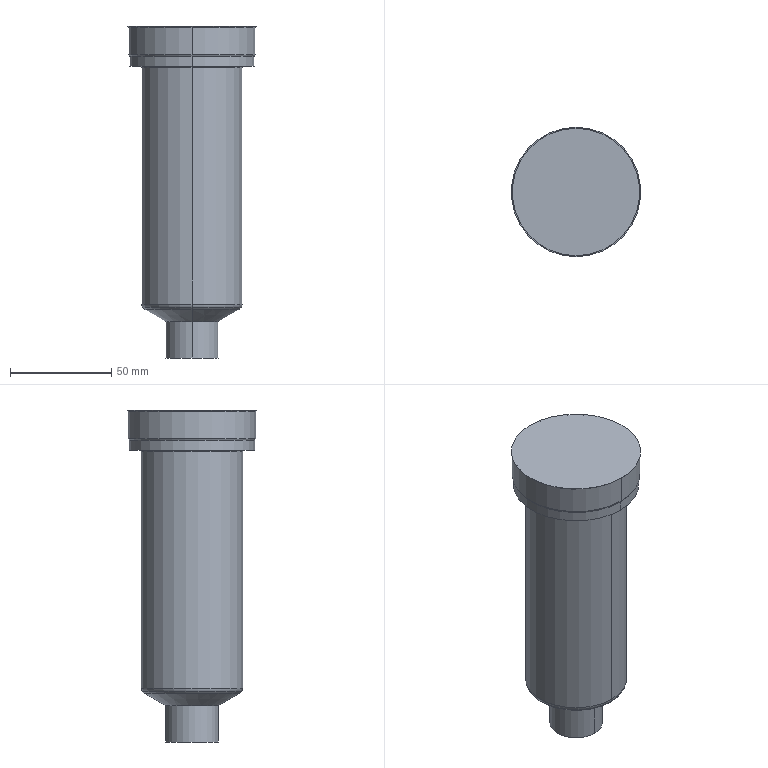Part | Creo | 1 solid | 23 faces | box 64 x 64 x 164.09 mm | volume 313430 mm3 | cylinder 8 | cone 8 | torus 4 | plane 3 | commonest cylinder face diameters 26 x2 50 x2 62 x2 63 x2
STEP:
#1=CARTESIAN_POINT('',(0.,48.,36.41));
#2=VERTEX_POINT('',#1);
#3=CARTESIAN_POINT('',(0.,22.,36.41));
#4=VERTEX_POINT('',#3);
#5=CARTESIAN_POINT('',(0.,35.,36.41));
#6=DIRECTION('',(0.,0.,-1.));
#7=DIRECTION('',(0.,1.,0.));
#8=AXIS2_PLACEMENT_3D('',#5,#6,#7);
#9=CIRCLE('',#8,13.);
#10=EDGE_CURVE('',#2,#4,#9,.T.);
#11=ORIENTED_EDGE('',*,*,#10,.F.);
#12=CARTESIAN_POINT('',(0.,35.,36.41));
#13=DIRECTION('',(0.,0.,-1.));
#14=DIRECTION('',(0.,-1.,0.));
#15=AXIS2_PLACEMENT_3D('',#12,#13,#14);
#16=CIRCLE('',#15,13.);
#17=EDGE_CURVE('',#4,#2,#16,.T.);
#18=ORIENTED_EDGE('',*,*,#17,.F.);
#19=EDGE_LOOP('',(#11,#18));
#20=FACE_OUTER_BOUND('',#19,.F.);
#21=CARTESIAN_POINT('',(1.,35.,36.41));
#22=DIRECTION('',(0.,0.,-1.));
#23=DIRECTION('',(0.,1.,0.));
#24=AXIS2_PLACEMENT_3D('',#21,#22,#23);
#25=PLANE('',#24);
#26=ADVANCED_FACE('',(#20),#25,.T.);
#27=CARTESIAN_POINT('',(0.,22.,54.41));
#28=VERTEX_POINT('',#27);
#29=CARTESIAN_POINT('',(0.,48.,54.41));
#30=VERTEX_POINT('',#29);
#31=CARTESIAN_POINT('',(0.,35.,54.41));
#32=DIRECTION('',(0.,0.,1.));
#33=DIRECTION('',(0.,-1.,0.));
#34=AXIS2_PLACEMENT_3D('',#31,#32,#33);
#35=CIRCLE('',#34,13.);
#36=EDGE_CURVE('',#28,#30,#35,.T.);
#37=ORIENTED_EDGE('',*,*,#36,.T.);
#38=CARTESIAN_POINT('',(0.,48.,54.41));
#39=DIRECTION('',(0.,0.,-1.));
#40=VECTOR('',#39,18.);
#41=LINE('',#38,#40);
#42=EDGE_CURVE('',#30,#2,#41,.T.);
#43=ORIENTED_EDGE('',*,*,#42,.T.);
#44=ORIENTED_EDGE('',*,*,#10,.T.);
#45=CARTESIAN_POINT('',(0.,22.,54.41));
#46=DIRECTION('',(0.,0.,-1.));
#47=VECTOR('',#46,18.);
#48=LINE('',#45,#47);
#49=EDGE_CURVE('',#28,#4,#48,.T.);
#50=ORIENTED_EDGE('',*,*,#49,.F.);
#51=EDGE_LOOP('',(#37,#43,#44,#50));
#52=FACE_OUTER_BOUND('',#51,.F.);
#53=CARTESIAN_POINT('',(0.,35.,36.41));
#54=DIRECTION('',(0.,0.,-1.));
#55=DIRECTION('',(0.,1.,0.));
#56=AXIS2_PLACEMENT_3D('',#53,#54,#55);
#57=CYLINDRICAL_SURFACE('',#56,13.);
#58=ADVANCED_FACE('',(#52),#57,.T.);
#59=CARTESIAN_POINT('',(0.,11.5,60.472));
#60=VERTEX_POINT('',#59);
#61=CARTESIAN_POINT('',(0.,58.5,60.472));
#62=VERTEX_POINT('',#61);
#63=CARTESIAN_POINT('',(0.,35.,60.472));
#64=DIRECTION('',(0.,0.,1.));
#65=DIRECTION('',(0.,-1.,0.));
#66=AXIS2_PLACEMENT_3D('',#63,#64,#65);
#67=CIRCLE('',#66,23.5);
#68=EDGE_CURVE('',#60,#62,#67,.T.);
#69=ORIENTED_EDGE('',*,*,#68,.T.);
#70=CARTESIAN_POINT('',(0.,48.,54.41));
#71=DIRECTION('',(0.,0.866,0.5));
#72=VECTOR('',#71,12.124);
#73=LINE('',#70,#72);
#74=EDGE_CURVE('',#30,#62,#73,.T.);
#75=ORIENTED_EDGE('',*,*,#74,.F.);
#76=ORIENTED_EDGE('',*,*,#36,.F.);
#77=CARTESIAN_POINT('',(0.,22.,54.41));
#78=DIRECTION('',(0.,-0.866,0.5));
#79=VECTOR('',#78,12.124);
#80=LINE('',#77,#79);
#81=EDGE_CURVE('',#28,#60,#80,.T.);
#82=ORIENTED_EDGE('',*,*,#81,.T.);
#83=EDGE_LOOP('',(#69,#75,#76,#82));
#84=FACE_OUTER_BOUND('',#83,.F.);
#85=CARTESIAN_POINT('',(0.,35.,57.441));
#86=DIRECTION('',(0.,0.,1.));
#87=DIRECTION('',(0.,-1.,0.));
#88=AXIS2_PLACEMENT_3D('',#85,#86,#87);
#89=CONICAL_SURFACE('',#88,18.25,60.);
#90=ADVANCED_FACE('',(#84),#89,.T.);
#91=ORIENTED_EDGE('',*,*,#68,.F.);
#92=CARTESIAN_POINT('',(0.,10.402,61.57));
#93=VERTEX_POINT('',#92);
#94=CARTESIAN_POINT('',(0.,13.,63.07));
#95=DIRECTION('',(1.,0.,0.));
#96=DIRECTION('',(0.,-0.866,-0.5));
#97=AXIS2_PLACEMENT_3D('',#94,#95,#96);
#98=CIRCLE('',#97,3.);
#99=EDGE_CURVE('',#93,#60,#98,.T.);
#100=ORIENTED_EDGE('',*,*,#99,.F.);
#101=CARTESIAN_POINT('',(0.,59.598,61.57));
#102=VERTEX_POINT('',#101);
#103=CARTESIAN_POINT('',(0.,35.,61.57));
#104=DIRECTION('',(0.,0.,-1.));
#105=DIRECTION('',(0.,1.,0.));
#106=AXIS2_PLACEMENT_3D('',#103,#104,#105);
#107=CIRCLE('',#106,24.598);
#108=EDGE_CURVE('',#102,#93,#107,.T.);
#109=ORIENTED_EDGE('',*,*,#108,.F.);
#110=CARTESIAN_POINT('',(0.,57.,63.07));
#111=DIRECTION('',(-1.,0.,0.));
#112=DIRECTION('',(0.,0.866,-0.5));
#113=AXIS2_PLACEMENT_3D('',#110,#111,#112);
#114=CIRCLE('',#113,3.);
#115=EDGE_CURVE('',#102,#62,#114,.T.);
#116=ORIENTED_EDGE('',*,*,#115,.T.);
#117=EDGE_LOOP('',(#91,#100,#109,#116));
#118=FACE_OUTER_BOUND('',#117,.F.);
#119=CARTESIAN_POINT('',(0.,35.,63.07));
#120=DIRECTION('',(0.,0.,-1.));
#121=DIRECTION('',(0.,1.,0.));
#122=AXIS2_PLACEMENT_3D('',#119,#120,#121);
#123=TOROIDAL_SURFACE('',#122,22.,3.);
#124=ADVANCED_FACE('',(#118),#123,.T.);
#125=CARTESIAN_POINT('',(0.,35.,60.472));
#126=DIRECTION('',(0.,0.,1.));
#127=DIRECTION('',(0.,1.,0.));
#128=AXIS2_PLACEMENT_3D('',#125,#126,#127);
#129=CIRCLE('',#128,23.5);
#130=EDGE_CURVE('',#62,#60,#129,.T.);
#131=ORIENTED_EDGE('',*,*,#130,.F.);
#132=ORIENTED_EDGE('',*,*,#115,.F.);
#133=CARTESIAN_POINT('',(0.,35.,61.57));
#134=DIRECTION('',(0.,0.,-1.));
#135=DIRECTION('',(0.,-1.,0.));
#136=AXIS2_PLACEMENT_3D('',#133,#134,#135);
#137=CIRCLE('',#136,24.598);
#138=EDGE_CURVE('',#93,#102,#137,.T.);
#139=ORIENTED_EDGE('',*,*,#138,.F.);
#140=ORIENTED_EDGE('',*,*,#99,.T.);
#141=EDGE_LOOP('',(#131,#132,#139,#140));
#142=FACE_OUTER_BOUND('',#141,.F.);
#143=CARTESIAN_POINT('',(0.,35.,63.07));
#144=DIRECTION('',(0.,0.,-1.));
#145=DIRECTION('',(0.,1.,0.));
#146=AXIS2_PLACEMENT_3D('',#143,#144,#145);
#147=TOROIDAL_SURFACE('',#146,22.,3.);
#148=ADVANCED_FACE('',(#142),#147,.T.);
#149=ORIENTED_EDGE('',*,*,#130,.T.);
#150=ORIENTED_EDGE('',*,*,#81,.F.);
#151=CARTESIAN_POINT('',(0.,35.,54.41));
#152=DIRECTION('',(0.,0.,1.));
#153=DIRECTION('',(0.,1.,0.));
#154=AXIS2_PLACEMENT_3D('',#151,#152,#153);
#155=CIRCLE('',#154,13.);
#156=EDGE_CURVE('',#30,#28,#155,.T.);
#157=ORIENTED_EDGE('',*,*,#156,.F.);
#158=ORIENTED_EDGE('',*,*,#74,.T.);
#159=EDGE_LOOP('',(#149,#150,#157,#158));
#160=FACE_OUTER_BOUND('',#159,.F.);
#161=CARTESIAN_POINT('',(0.,35.,57.441));
#162=DIRECTION('',(0.,0.,1.));
#163=DIRECTION('',(0.,-1.,0.));
#164=AXIS2_PLACEMENT_3D('',#161,#162,#163);
#165=CONICAL_SURFACE('',#164,18.25,60.);
#166=ADVANCED_FACE('',(#160),#165,.T.);
#167=ORIENTED_EDGE('',*,*,#156,.T.);
#168=ORIENTED_EDGE('',*,*,#49,.T.);
#169=ORIENTED_EDGE('',*,*,#17,.T.);
#170=ORIENTED_EDGE('',*,*,#42,.F.);
#171=EDGE_LOOP('',(#167,#168,#169,#170));
#172=FACE_OUTER_BOUND('',#171,.F.);
#173=CARTESIAN_POINT('',(0.,35.,36.41));
#174=DIRECTION('',(0.,0.,-1.));
#175=DIRECTION('',(0.,1.,0.));
#176=AXIS2_PLACEMENT_3D('',#173,#174,#175);
#177=CYLINDRICAL_SURFACE('',#176,13.);
#178=ADVANCED_FACE('',(#172),#177,.T.);
#179=CARTESIAN_POINT('',(0.,10.,63.07));
#180=VERTEX_POINT('',#179);
#181=CARTESIAN_POINT('',(0.,60.,63.07));
#182=VERTEX_POINT('',#181);
#183=CARTESIAN_POINT('',(0.,35.,63.07));
#184=DIRECTION('',(0.,0.,-1.));
#185=DIRECTION('',(0.,-1.,0.));
#186=AXIS2_PLACEMENT_3D('',#183,#184,#185);
#187=CIRCLE('',#186,25.);
#188=EDGE_CURVE('',#180,#182,#187,.T.);
#189=ORIENTED_EDGE('',*,*,#188,.F.);
#190=CARTESIAN_POINT('',(0.,13.,63.07));
#191=DIRECTION('',(1.,0.,0.));
#192=DIRECTION('',(0.,-1.,0.));
#193=AXIS2_PLACEMENT_3D('',#190,#191,#192);
#194=CIRCLE('',#193,3.);
#195=EDGE_CURVE('',#180,#93,#194,.T.);
#196=ORIENTED_EDGE('',*,*,#195,.T.);
#197=ORIENTED_EDGE('',*,*,#138,.T.);
#198=CARTESIAN_POINT('',(0.,57.,63.07));
#199=DIRECTION('',(-1.,0.,0.));
#200=DIRECTION('',(0.,1.,0.));
#201=AXIS2_PLACEMENT_3D('',#198,#199,#200);
#202=CIRCLE('',#201,3.);
#203=EDGE_CURVE('',#182,#102,#202,.T.);
#204=ORIENTED_EDGE('',*,*,#203,.F.);
#205=EDGE_LOOP('',(#189,#196,#197,#204));
#206=FACE_OUTER_BOUND('',#205,.F.);
#207=CARTESIAN_POINT('',(0.,35.,63.07));
#208=DIRECTION('',(0.,0.,-1.));
#209=DIRECTION('',(0.,1.,0.));
#210=AXIS2_PLACEMENT_3D('',#207,#208,#209);
#211=TOROIDAL_SURFACE('',#210,22.,3.);
#212=ADVANCED_FACE('',(#206),#211,.T.);
#213=CARTESIAN_POINT('',(0.,60.,180.));
#214=VERTEX_POINT('',#213);
#215=CARTESIAN_POINT('',(0.,10.,180.));
#216=VERTEX_POINT('',#215);
#217=CARTESIAN_POINT('',(0.,35.,180.));
#218=DIRECTION('',(0.,0.,1.));
#219=DIRECTION('',(0.,1.,0.));
#220=AXIS2_PLACEMENT_3D('',#217,#218,#219);
#221=CIRCLE('',#220,25.);
#222=EDGE_CURVE('',#214,#216,#221,.T.);
#223=ORIENTED_EDGE('',*,*,#222,.T.);
#224=CARTESIAN_POINT('',(0.,10.,180.));
#225=DIRECTION('',(0.,0.,-1.));
#226=VECTOR('',#225,116.93);
#227=LINE('',#224,#226);
#228=EDGE_CURVE('',#216,#180,#227,.T.);
#229=ORIENTED_EDGE('',*,*,#228,.T.);
#230=ORIENTED_EDGE('',*,*,#188,.T.);
#231=CARTESIAN_POINT('',(0.,60.,180.));
#232=DIRECTION('',(0.,0.,-1.));
#233=VECTOR('',#232,116.93);
#234=LINE('',#231,#233);
#235=EDGE_CURVE('',#214,#182,#234,.T.);
#236=ORIENTED_EDGE('',*,*,#235,.F.);
#237=EDGE_LOOP('',(#223,#229,#230,#236));
#238=FACE_OUTER_BOUND('',#237,.F.);
#239=CARTESIAN_POINT('',(0.,35.,36.41));
#240=DIRECTION('',(0.,0.,-1.));
#241=DIRECTION('',(0.,1.,0.));
#242=AXIS2_PLACEMENT_3D('',#239,#240,#241);
#243=CYLINDRICAL_SURFACE('',#242,25.);
#244=ADVANCED_FACE('',(#238),#243,.T.);
#245=CARTESIAN_POINT('',(0.,60.5,180.5));
#246=VERTEX_POINT('',#245);
#247=CARTESIAN_POINT('',(0.,9.5,180.5));
#248=VERTEX_POINT('',#247);
#249=CARTESIAN_POINT('',(0.,35.,180.5));
#250=DIRECTION('',(0.,0.,1.));
#251=DIRECTION('',(0.,1.,0.));
#252=AXIS2_PLACEMENT_3D('',#249,#250,#251);
#253=CIRCLE('',#252,25.5);
#254=EDGE_CURVE('',#246,#248,#253,.T.);
#255=ORIENTED_EDGE('',*,*,#254,.T.);
#256=CARTESIAN_POINT('',(0.,10.,180.));
#257=DIRECTION('',(0.,-0.7071,0.7071));
#258=VECTOR('',#257,0.7071);
#259=LINE('',#256,#258);
#260=EDGE_CURVE('',#216,#248,#259,.T.);
#261=ORIENTED_EDGE('',*,*,#260,.F.);
#262=ORIENTED_EDGE('',*,*,#222,.F.);
#263=CARTESIAN_POINT('',(0.,60.,180.));
#264=DIRECTION('',(0.,0.7071,0.7071));
#265=VECTOR('',#264,0.7071);
#266=LINE('',#263,#265);
#267=EDGE_CURVE('',#214,#246,#266,.T.);
#268=ORIENTED_EDGE('',*,*,#267,.T.);
#269=EDGE_LOOP('',(#255,#261,#262,#268));
#270=FACE_OUTER_BOUND('',#269,.F.);
#271=CARTESIAN_POINT('',(0.,35.,180.25));
#272=DIRECTION('',(0.,0.,1.));
#273=DIRECTION('',(0.,-1.,0.));
#274=AXIS2_PLACEMENT_3D('',#271,#272,#273);
#275=CONICAL_SURFACE('',#274,25.25,45.);
#276=ADVANCED_FACE('',(#270),#275,.T.);
#277=CARTESIAN_POINT('',(0.,66.,180.5));
#278=VERTEX_POINT('',#277);
#279=CARTESIAN_POINT('',(0.,4.,180.5));
#280=VERTEX_POINT('',#279);
#281=CARTESIAN_POINT('',(0.,35.,180.5));
#282=DIRECTION('',(0.,0.,-1.));
#283=DIRECTION('',(0.,1.,0.));
#284=AXIS2_PLACEMENT_3D('',#281,#282,#283);
#285=CIRCLE('',#284,31.);
#286=EDGE_CURVE('',#278,#280,#285,.T.);
#287=ORIENTED_EDGE('',*,*,#286,.F.);
#288=CARTESIAN_POINT('',(0.,35.,180.5));
#289=DIRECTION('',(0.,0.,-1.));
#290=DIRECTION('',(0.,-1.,0.));
#291=AXIS2_PLACEMENT_3D('',#288,#289,#290);
#292=CIRCLE('',#291,31.);
#293=EDGE_CURVE('',#280,#278,#292,.T.);
#294=ORIENTED_EDGE('',*,*,#293,.F.);
#295=EDGE_LOOP('',(#287,#294));
#296=FACE_OUTER_BOUND('',#295,.F.);
#297=ORIENTED_EDGE('',*,*,#254,.F.);
#298=CARTESIAN_POINT('',(0.,35.,180.5));
#299=DIRECTION('',(0.,0.,1.));
#300=DIRECTION('',(0.,-1.,0.));
#301=AXIS2_PLACEMENT_3D('',#298,#299,#300);
#302=CIRCLE('',#301,25.5);
#303=EDGE_CURVE('',#248,#246,#302,.T.);
#304=ORIENTED_EDGE('',*,*,#303,.F.);
#305=EDGE_LOOP('',(#297,#304));
#306=FACE_BOUND('',#305,.F.);
#307=CARTESIAN_POINT('',(25.5,35.,180.5));
#308=DIRECTION('',(0.,0.,-1.));
#309=DIRECTION('',(0.,1.,0.));
#310=AXIS2_PLACEMENT_3D('',#307,#308,#309);
#311=PLANE('',#310);
#312=ADVANCED_FACE('',(#296,#306),#311,.T.);
#313=CARTESIAN_POINT('',(0.,4.,185.5));
#314=VERTEX_POINT('',#313);
#315=CARTESIAN_POINT('',(0.,66.,185.5));
#316=VERTEX_POINT('',#315);
#317=CARTESIAN_POINT('',(0.,35.,185.5));
#318=DIRECTION('',(0.,0.,1.));
#319=DIRECTION('',(0.,-1.,0.));
#320=AXIS2_PLACEMENT_3D('',#317,#318,#319);
#321=CIRCLE('',#320,31.);
#322=EDGE_CURVE('',#314,#316,#321,.T.);
#323=ORIENTED_EDGE('',*,*,#322,.T.);
#324=CARTESIAN_POINT('',(0.,66.,185.5));
#325=DIRECTION('',(0.,0.,-1.));
#326=VECTOR('',#325,5.);
#327=LINE('',#324,#326);
#328=EDGE_CURVE('',#316,#278,#327,.T.);
#329=ORIENTED_EDGE('',*,*,#328,.T.);
#330=ORIENTED_EDGE('',*,*,#286,.T.);
#331=CARTESIAN_POINT('',(0.,4.,185.5));
#332=DIRECTION('',(0.,0.,-1.));
#333=VECTOR('',#332,5.);
#334=LINE('',#331,#333);
#335=EDGE_CURVE('',#314,#280,#334,.T.);
#336=ORIENTED_EDGE('',*,*,#335,.F.);
#337=EDGE_LOOP('',(#323,#329,#330,#336));
#338=FACE_OUTER_BOUND('',#337,.F.);
#339=CARTESIAN_POINT('',(0.,35.,36.41));
#340=DIRECTION('',(0.,0.,-1.));
#341=DIRECTION('',(0.,1.,0.));
#342=AXIS2_PLACEMENT_3D('',#339,#340,#341);
#343=CYLINDRICAL_SURFACE('',#342,31.);
#344=ADVANCED_FACE('',(#338),#343,.T.);
#345=CARTESIAN_POINT('',(0.,66.5,186.366));
#346=VERTEX_POINT('',#345);
#347=CARTESIAN_POINT('',(0.,3.5,186.366));
#348=VERTEX_POINT('',#347);
#349=CARTESIAN_POINT('',(0.,35.,186.366));
#350=DIRECTION('',(0.,0.,-1.));
#351=DIRECTION('',(0.,1.,0.));
#352=AXIS2_PLACEMENT_3D('',#349,#350,#351);
#353=CIRCLE('',#352,31.5);
#354=EDGE_CURVE('',#346,#348,#353,.T.);
#355=ORIENTED_EDGE('',*,*,#354,.F.);
#356=CARTESIAN_POINT('',(0.,66.,185.5));
#357=DIRECTION('',(0.,0.5,0.866));
#358=VECTOR('',#357,1.);
#359=LINE('',#356,#358);
#360=EDGE_CURVE('',#316,#346,#359,.T.);
#361=ORIENTED_EDGE('',*,*,#360,.F.);
#362=ORIENTED_EDGE('',*,*,#322,.F.);
#363=CARTESIAN_POINT('',(0.,4.,185.5));
#364=DIRECTION('',(0.,-0.5,0.866));
#365=VECTOR('',#364,1.);
#366=LINE('',#363,#365);
#367=EDGE_CURVE('',#314,#348,#366,.T.);
#368=ORIENTED_EDGE('',*,*,#367,.T.);
#369=EDGE_LOOP('',(#355,#361,#362,#368));
#370=FACE_OUTER_BOUND('',#369,.F.);
#371=CARTESIAN_POINT('',(0.,35.,185.933));
#372=DIRECTION('',(0.,0.,1.));
#373=DIRECTION('',(0.,-1.,0.));
#374=AXIS2_PLACEMENT_3D('',#371,#372,#373);
#375=CONICAL_SURFACE('',#374,31.25,30.);
#376=ADVANCED_FACE('',(#370),#375,.T.);
#377=CARTESIAN_POINT('',(0.,3.5,200.));
#378=VERTEX_POINT('',#377);
#379=CARTESIAN_POINT('',(0.,66.5,200.));
#380=VERTEX_POINT('',#379);
#381=CARTESIAN_POINT('',(0.,35.,200.));
#382=DIRECTION('',(0.,0.,1.));
#383=DIRECTION('',(0.,-1.,0.));
#384=AXIS2_PLACEMENT_3D('',#381,#382,#383);
#385=CIRCLE('',#384,31.5);
#386=EDGE_CURVE('',#378,#380,#385,.T.);
#387=ORIENTED_EDGE('',*,*,#386,.T.);
#388=CARTESIAN_POINT('',(0.,66.5,200.));
#389=DIRECTION('',(0.,0.,-1.));
#390=VECTOR('',#389,13.634);
#391=LINE('',#388,#390);
#392=EDGE_CURVE('',#380,#346,#391,.T.);
#393=ORIENTED_EDGE('',*,*,#392,.T.);
#394=ORIENTED_EDGE('',*,*,#354,.T.);
#395=CARTESIAN_POINT('',(0.,3.5,200.));
#396=DIRECTION('',(0.,0.,-1.));
#397=VECTOR('',#396,13.634);
#398=LINE('',#395,#397);
#399=EDGE_CURVE('',#378,#348,#398,.T.);
#400=ORIENTED_EDGE('',*,*,#399,.F.);
#401=EDGE_LOOP('',(#387,#393,#394,#400));
#402=FACE_OUTER_BOUND('',#401,.F.);
#403=CARTESIAN_POINT('',(0.,35.,36.41));
#404=DIRECTION('',(0.,0.,-1.));
#405=DIRECTION('',(0.,1.,0.));
#406=AXIS2_PLACEMENT_3D('',#403,#404,#405);
#407=CYLINDRICAL_SURFACE('',#406,31.5);
#408=ADVANCED_FACE('',(#402),#407,.T.);
#409=CARTESIAN_POINT('',(0.,3.,200.5));
#410=VERTEX_POINT('',#409);
#411=CARTESIAN_POINT('',(0.,67.,200.5));
#412=VERTEX_POINT('',#411);
#413=CARTESIAN_POINT('',(0.,35.,200.5));
#414=DIRECTION('',(0.,0.,1.));
#415=DIRECTION('',(0.,-1.,0.));
#416=AXIS2_PLACEMENT_3D('',#413,#414,#415);
#417=CIRCLE('',#416,32.);
#418=EDGE_CURVE('',#410,#412,#417,.T.);
#419=ORIENTED_EDGE('',*,*,#418,.T.);
#420=CARTESIAN_POINT('',(0.,66.5,200.));
#421=DIRECTION('',(0.,0.7071,0.7071));
#422=VECTOR('',#421,0.7071);
#423=LINE('',#420,#422);
#424=EDGE_CURVE('',#380,#412,#423,.T.);
#425=ORIENTED_EDGE('',*,*,#424,.F.);
#426=ORIENTED_EDGE('',*,*,#386,.F.);
#427=CARTESIAN_POINT('',(0.,3.5,200.));
#428=DIRECTION('',(0.,-0.7071,0.7071));
#429=VECTOR('',#428,0.7071);
#430=LINE('',#427,#429);
#431=EDGE_CURVE('',#378,#410,#430,.T.);
#432=ORIENTED_EDGE('',*,*,#431,.T.);
#433=EDGE_LOOP('',(#419,#425,#426,#432));
#434=FACE_OUTER_BOUND('',#433,.F.);
#435=CARTESIAN_POINT('',(0.,35.,200.25));
#436=DIRECTION('',(0.,0.,1.));
#437=DIRECTION('',(0.,-1.,0.));
#438=AXIS2_PLACEMENT_3D('',#435,#436,#437);
#439=CONICAL_SURFACE('',#438,31.75,45.);
#440=ADVANCED_FACE('',(#434),#439,.T.);
#441=CARTESIAN_POINT('',(0.,35.,200.5));
#442=DIRECTION('',(0.,0.,1.));
#443=DIRECTION('',(0.,1.,0.));
#444=AXIS2_PLACEMENT_3D('',#441,#442,#443);
#445=CIRCLE('',#444,32.);
#446=EDGE_CURVE('',#412,#410,#445,.T.);
#447=ORIENTED_EDGE('',*,*,#446,.F.);
#448=ORIENTED_EDGE('',*,*,#418,.F.);
#449=EDGE_LOOP('',(#447,#448));
#450=FACE_OUTER_BOUND('',#449,.F.);
#451=CARTESIAN_POINT('',(32.,35.,200.5));
#452=DIRECTION('',(0.,0.,1.));
#453=DIRECTION('',(0.,-1.,0.));
#454=AXIS2_PLACEMENT_3D('',#451,#452,#453);
#455=PLANE('',#454);
#456=ADVANCED_FACE('',(#450),#455,.T.);
#457=ORIENTED_EDGE('',*,*,#446,.T.);
#458=ORIENTED_EDGE('',*,*,#431,.F.);
#459=CARTESIAN_POINT('',(0.,35.,200.));
#460=DIRECTION('',(0.,0.,1.));
#461=DIRECTION('',(0.,1.,0.));
#462=AXIS2_PLACEMENT_3D('',#459,#460,#461);
#463=CIRCLE('',#462,31.5);
#464=EDGE_CURVE('',#380,#378,#463,.T.);
#465=ORIENTED_EDGE('',*,*,#464,.F.);
#466=ORIENTED_EDGE('',*,*,#424,.T.);
#467=EDGE_LOOP('',(#457,#458,#465,#466));
#468=FACE_OUTER_BOUND('',#467,.F.);
#469=CARTESIAN_POINT('',(0.,35.,200.25));
#470=DIRECTION('',(0.,0.,1.));
#471=DIRECTION('',(0.,-1.,0.));
#472=AXIS2_PLACEMENT_3D('',#469,#470,#471);
#473=CONICAL_SURFACE('',#472,31.75,45.);
#474=ADVANCED_FACE('',(#468),#473,.T.);
#475=ORIENTED_EDGE('',*,*,#464,.T.);
#476=ORIENTED_EDGE('',*,*,#399,.T.);
#477=CARTESIAN_POINT('',(0.,35.,186.366));
#478=DIRECTION('',(0.,0.,-1.));
#479=DIRECTION('',(0.,-1.,0.));
#480=AXIS2_PLACEMENT_3D('',#477,#478,#479);
#481=CIRCLE('',#480,31.5);
#482=EDGE_CURVE('',#348,#346,#481,.T.);
#483=ORIENTED_EDGE('',*,*,#482,.T.);
#484=ORIENTED_EDGE('',*,*,#392,.F.);
#485=EDGE_LOOP('',(#475,#476,#483,#484));
#486=FACE_OUTER_BOUND('',#485,.F.);
#487=CARTESIAN_POINT('',(0.,35.,36.41));
#488=DIRECTION('',(0.,0.,-1.));
#489=DIRECTION('',(0.,1.,0.));
#490=AXIS2_PLACEMENT_3D('',#487,#488,#489);
#491=CYLINDRICAL_SURFACE('',#490,31.5);
#492=ADVANCED_FACE('',(#486),#491,.T.);
#493=ORIENTED_EDGE('',*,*,#482,.F.);
#494=ORIENTED_EDGE('',*,*,#367,.F.);
#495=CARTESIAN_POINT('',(0.,35.,185.5));
#496=DIRECTION('',(0.,0.,1.));
#497=DIRECTION('',(0.,1.,0.));
#498=AXIS2_PLACEMENT_3D('',#495,#496,#497);
#499=CIRCLE('',#498,31.);
#500=EDGE_CURVE('',#316,#314,#499,.T.);
#501=ORIENTED_EDGE('',*,*,#500,.F.);
#502=ORIENTED_EDGE('',*,*,#360,.T.);
#503=EDGE_LOOP('',(#493,#494,#501,#502));
#504=FACE_OUTER_BOUND('',#503,.F.);
#505=CARTESIAN_POINT('',(0.,35.,185.933));
#506=DIRECTION('',(0.,0.,1.));
#507=DIRECTION('',(0.,-1.,0.));
#508=AXIS2_PLACEMENT_3D('',#505,#506,#507);
#509=CONICAL_SURFACE('',#508,31.25,30.);
#510=ADVANCED_FACE('',(#504),#509,.T.);
#511=ORIENTED_EDGE('',*,*,#500,.T.);
#512=ORIENTED_EDGE('',*,*,#335,.T.);
#513=ORIENTED_EDGE('',*,*,#293,.T.);
#514=ORIENTED_EDGE('',*,*,#328,.F.);
#515=EDGE_LOOP('',(#511,#512,#513,#514));
#516=FACE_OUTER_BOUND('',#515,.F.);
#517=CARTESIAN_POINT('',(0.,35.,36.41));
#518=DIRECTION('',(0.,0.,-1.));
#519=DIRECTION('',(0.,1.,0.));
#520=AXIS2_PLACEMENT_3D('',#517,#518,#519);
#521=CYLINDRICAL_SURFACE('',#520,31.);
#522=ADVANCED_FACE('',(#516),#521,.T.);
#523=ORIENTED_EDGE('',*,*,#303,.T.);
#524=ORIENTED_EDGE('',*,*,#267,.F.);
#525=CARTESIAN_POINT('',(0.,35.,180.));
#526=DIRECTION('',(0.,0.,1.));
#527=DIRECTION('',(0.,-1.,0.));
#528=AXIS2_PLACEMENT_3D('',#525,#526,#527);
#529=CIRCLE('',#528,25.);
#530=EDGE_CURVE('',#216,#214,#529,.T.);
#531=ORIENTED_EDGE('',*,*,#530,.F.);
#532=ORIENTED_EDGE('',*,*,#260,.T.);
#533=EDGE_LOOP('',(#523,#524,#531,#532));
#534=FACE_OUTER_BOUND('',#533,.F.);
#535=CARTESIAN_POINT('',(0.,35.,180.25));
#536=DIRECTION('',(0.,0.,1.));
#537=DIRECTION('',(0.,-1.,0.));
#538=AXIS2_PLACEMENT_3D('',#535,#536,#537);
#539=CONICAL_SURFACE('',#538,25.25,45.);
#540=ADVANCED_FACE('',(#534),#539,.T.);
#541=ORIENTED_EDGE('',*,*,#530,.T.);
#542=ORIENTED_EDGE('',*,*,#235,.T.);
#543=CARTESIAN_POINT('',(0.,35.,63.07));
#544=DIRECTION('',(0.,0.,-1.));
#545=DIRECTION('',(0.,1.,0.));
#546=AXIS2_PLACEMENT_3D('',#543,#544,#545);
#547=CIRCLE('',#546,25.);
#548=EDGE_CURVE('',#182,#180,#547,.T.);
#549=ORIENTED_EDGE('',*,*,#548,.T.);
#550=ORIENTED_EDGE('',*,*,#228,.F.);
#551=EDGE_LOOP('',(#541,#542,#549,#550));
#552=FACE_OUTER_BOUND('',#551,.F.);
#553=CARTESIAN_POINT('',(0.,35.,36.41));
#554=DIRECTION('',(0.,0.,-1.));
#555=DIRECTION('',(0.,1.,0.));
#556=AXIS2_PLACEMENT_3D('',#553,#554,#555);
#557=CYLINDRICAL_SURFACE('',#556,25.);
#558=ADVANCED_FACE('',(#552),#557,.T.);
#559=ORIENTED_EDGE('',*,*,#548,.F.);
#560=ORIENTED_EDGE('',*,*,#203,.T.);
#561=ORIENTED_EDGE('',*,*,#108,.T.);
#562=ORIENTED_EDGE('',*,*,#195,.F.);
#563=EDGE_LOOP('',(#559,#560,#561,#562));
#564=FACE_OUTER_BOUND('',#563,.F.);
#565=CARTESIAN_POINT('',(0.,35.,63.07));
#566=DIRECTION('',(0.,0.,-1.));
#567=DIRECTION('',(0.,1.,0.));
#568=AXIS2_PLACEMENT_3D('',#565,#566,#567);
#569=TOROIDAL_SURFACE('',#568,22.,3.);
#570=ADVANCED_FACE('',(#564),#569,.T.);
#571=CLOSED_SHELL('',(#26,#58,#90,#124,#148,#166,#178,#212,#244,#276,#312,#344,#376,#408,#440,#456,#474,#492,#510,#522,#540,#558,#570));
#572=MANIFOLD_SOLID_BREP('',#571);
#573=(LENGTH_UNIT()NAMED_UNIT(*)SI_UNIT(.MILLI.,.METRE.));
#574=UNCERTAINTY_MEASURE_WITH_UNIT(LENGTH_MEASURE(0.01874),#573,'','');
#575=(NAMED_UNIT(*)PLANE_ANGLE_UNIT()SI_UNIT($,.RADIAN.));
#576=PLANE_ANGLE_MEASURE_WITH_UNIT(PLANE_ANGLE_MEASURE(0.01745),#575);
#577=(CONVERSION_BASED_UNIT('DEGREE',#576)NAMED_UNIT(*)PLANE_ANGLE_UNIT());
#578=(NAMED_UNIT(*)SI_UNIT($,.STERADIAN.)SOLID_ANGLE_UNIT());
#579=(GEOMETRIC_REPRESENTATION_CONTEXT(3)GLOBAL_UNCERTAINTY_ASSIGNED_CONTEXT((#574))GLOBAL_UNIT_ASSIGNED_CONTEXT((#573,#577,#578))REPRESENTATION_CONTEXT('',''));
#580=ADVANCED_BREP_SHAPE_REPRESENTATION('',(#572),#579);